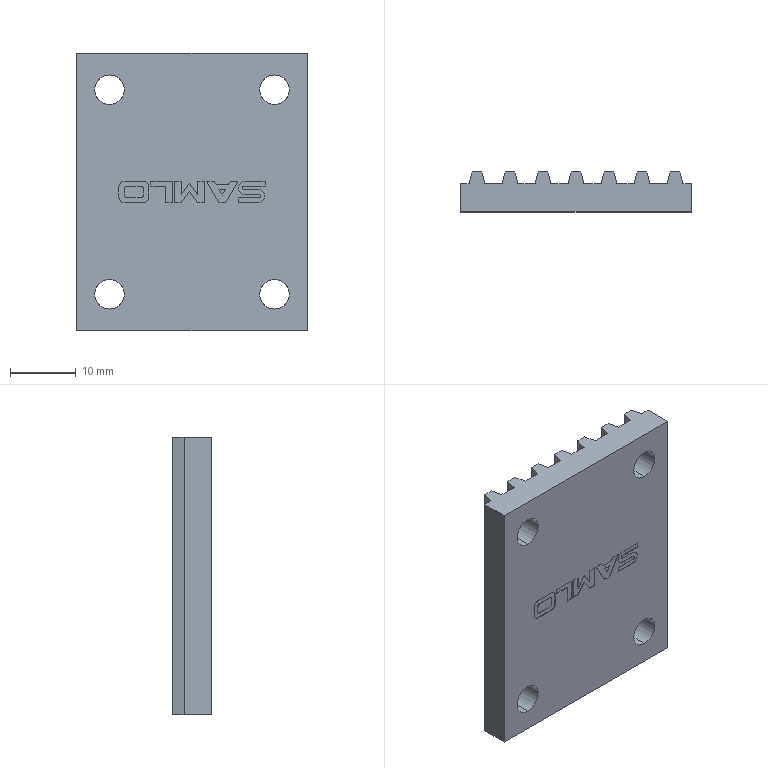Part | SolidWorks | features BaseBody 1 | 1 solid | 118 faces | box 35 x 6 x 42 mm | volume 6903 mm3 | plane 98 | cylinder 20 | commonest cylinder face diameters 4.5 x8 0.75 x4 1.59 x4 0.538 x2 1.972 x2